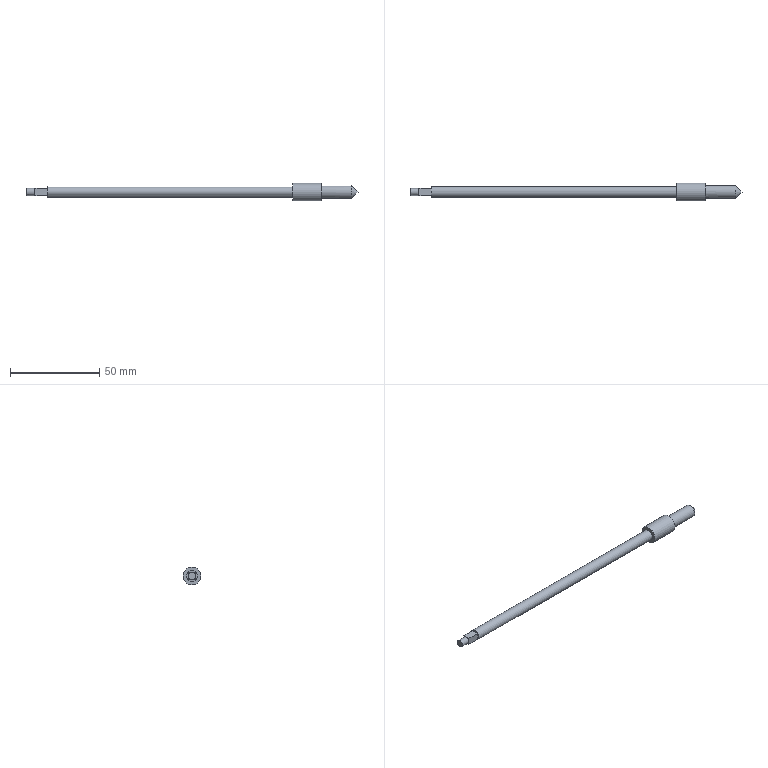Part | STEP file | 1-23.5 | 1 solid | 17 faces | box 185.5 x 10 x 10 mm | volume 6004 mm3 | plane 12 | cylinder 4 | cone 1 | commonest cylinder face diameters 4 x1 6 x1 7 x1 10 x1
STEP:
#1=CARTESIAN_POINT('',(0.,0.,0.));
#2=DIRECTION('',(0.,0.,1.));
#3=DIRECTION('',(1.,0.,0.));
#4=AXIS2_PLACEMENT_3D('',#1,#2,#3);
#5=CARTESIAN_POINT('',(0.,5.,0.));
#6=VERTEX_POINT('',#5);
#7=CARTESIAN_POINT('',(-16.,5.,0.));
#8=VERTEX_POINT('',#7);
#9=CARTESIAN_POINT('',(0.,5.,0.));
#10=DIRECTION('',(-1.,0.,0.));
#11=VECTOR('',#10,1.);
#12=LINE('',#9,#11);
#13=CARTESIAN_POINT('',(0.,0.,0.));
#14=DIRECTION('',(-1.,0.,0.));
#15=DIRECTION('',(0.,1.,0.));
#16=AXIS2_PLACEMENT_3D('',#13,#14,#15);
#17=CYLINDRICAL_SURFACE('',#16,5.);
#18=CARTESIAN_POINT('',(6.283,0.));
#19=DIRECTION('',(0.,1.));
#20=VECTOR('',#19,1.);
#21=LINE('',#18,#20);
#22=(GEOMETRIC_REPRESENTATION_CONTEXT(2)PARAMETRIC_REPRESENTATION_CONTEXT()REPRESENTATION_CONTEXT('',''));
#23=DEFINITIONAL_REPRESENTATION('',(#21),#22);
#24=PCURVE('',#17,#23);
#25=CARTESIAN_POINT('',(0.,0.));
#26=DIRECTION('',(0.,1.));
#27=VECTOR('',#26,1.);
#28=LINE('',#25,#27);
#29=(GEOMETRIC_REPRESENTATION_CONTEXT(2)PARAMETRIC_REPRESENTATION_CONTEXT()REPRESENTATION_CONTEXT('',''));
#30=DEFINITIONAL_REPRESENTATION('',(#28),#29);
#31=PCURVE('',#17,#30);
#32=SEAM_CURVE('',#12,(#24,#31),.PCURVE_S1.);
#33=EDGE_CURVE('',#6,#8,#32,.T.);
#34=ORIENTED_EDGE('',*,*,#33,.T.);
#35=CARTESIAN_POINT('',(-16.,0.,0.));
#36=DIRECTION('',(1.,0.,0.));
#37=DIRECTION('',(0.,1.,0.));
#38=AXIS2_PLACEMENT_3D('',#35,#36,#37);
#39=CIRCLE('',#38,5.);
#40=CARTESIAN_POINT('',(6.283,16.));
#41=DIRECTION('',(-1.,0.));
#42=VECTOR('',#41,1.);
#43=LINE('',#40,#42);
#44=(GEOMETRIC_REPRESENTATION_CONTEXT(2)PARAMETRIC_REPRESENTATION_CONTEXT()REPRESENTATION_CONTEXT('',''));
#45=DEFINITIONAL_REPRESENTATION('',(#43),#44);
#46=PCURVE('',#17,#45);
#47=CARTESIAN_POINT('',(-16.,-1.34,0.));
#48=DIRECTION('',(1.,0.,0.));
#49=DIRECTION('',(0.,0.,-1.));
#50=AXIS2_PLACEMENT_3D('',#47,#48,#49);
#51=PLANE('',#50);
#52=CARTESIAN_POINT('',(0.,1.34));
#53=DIRECTION('',(0.,1.));
#54=AXIS2_PLACEMENT_2D('',#52,#53);
#55=CIRCLE('',#54,5.);
#56=(GEOMETRIC_REPRESENTATION_CONTEXT(2)PARAMETRIC_REPRESENTATION_CONTEXT()REPRESENTATION_CONTEXT('',''));
#57=DEFINITIONAL_REPRESENTATION('',(#55),#56);
#58=PCURVE('',#51,#57);
#59=SURFACE_CURVE('',#39,(#46,#58),.PCURVE_S1.);
#60=EDGE_CURVE('',#8,#8,#59,.T.);
#61=ORIENTED_EDGE('',*,*,#60,.T.);
#62=ORIENTED_EDGE('',*,*,#33,.F.);
#63=CARTESIAN_POINT('',(0.,0.,0.));
#64=DIRECTION('',(1.,0.,0.));
#65=DIRECTION('',(0.,1.,0.));
#66=AXIS2_PLACEMENT_3D('',#63,#64,#65);
#67=CIRCLE('',#66,5.);
#68=CARTESIAN_POINT('',(6.283,0.));
#69=DIRECTION('',(-1.,0.));
#70=VECTOR('',#69,1.);
#71=LINE('',#68,#70);
#72=(GEOMETRIC_REPRESENTATION_CONTEXT(2)PARAMETRIC_REPRESENTATION_CONTEXT()REPRESENTATION_CONTEXT('',''));
#73=DEFINITIONAL_REPRESENTATION('',(#71),#72);
#74=PCURVE('',#17,#73);
#75=CARTESIAN_POINT('',(0.,-1.34,0.));
#76=DIRECTION('',(1.,0.,0.));
#77=DIRECTION('',(0.,0.,-1.));
#78=AXIS2_PLACEMENT_3D('',#75,#76,#77);
#79=PLANE('',#78);
#80=CARTESIAN_POINT('',(0.,1.34));
#81=DIRECTION('',(0.,1.));
#82=AXIS2_PLACEMENT_2D('',#80,#81);
#83=CIRCLE('',#82,5.);
#84=(GEOMETRIC_REPRESENTATION_CONTEXT(2)PARAMETRIC_REPRESENTATION_CONTEXT()REPRESENTATION_CONTEXT('',''));
#85=DEFINITIONAL_REPRESENTATION('',(#83),#84);
#86=PCURVE('',#79,#85);
#87=SURFACE_CURVE('',#67,(#74,#86),.PCURVE_S1.);
#88=EDGE_CURVE('',#6,#6,#87,.T.);
#89=ORIENTED_EDGE('',*,*,#88,.F.);
#90=EDGE_LOOP('',(#34,#61,#62,#89));
#91=FACE_BOUND('',#90,.T.);
#92=ADVANCED_FACE('',(#91),#17,.T.);
#93=ORIENTED_EDGE('',*,*,#88,.T.);
#94=EDGE_LOOP('',(#93));
#95=FACE_BOUND('',#94,.T.);
#96=CARTESIAN_POINT('',(0.,3.5,0.));
#97=VERTEX_POINT('',#96);
#98=CARTESIAN_POINT('',(0.,0.,0.));
#99=DIRECTION('',(1.,0.,0.));
#100=DIRECTION('',(0.,1.,0.));
#101=AXIS2_PLACEMENT_3D('',#98,#99,#100);
#102=CIRCLE('',#101,3.5);
#103=CARTESIAN_POINT('',(0.,1.34));
#104=DIRECTION('',(0.,1.));
#105=AXIS2_PLACEMENT_2D('',#103,#104);
#106=CIRCLE('',#105,3.5);
#107=(GEOMETRIC_REPRESENTATION_CONTEXT(2)PARAMETRIC_REPRESENTATION_CONTEXT()REPRESENTATION_CONTEXT('',''));
#108=DEFINITIONAL_REPRESENTATION('',(#106),#107);
#109=PCURVE('',#79,#108);
#110=CARTESIAN_POINT('',(0.,0.,0.));
#111=DIRECTION('',(1.,0.,0.));
#112=DIRECTION('',(0.,1.,0.));
#113=AXIS2_PLACEMENT_3D('',#110,#111,#112);
#114=CYLINDRICAL_SURFACE('',#113,3.5);
#115=CARTESIAN_POINT('',(0.,0.));
#116=DIRECTION('',(1.,0.));
#117=VECTOR('',#116,1.);
#118=LINE('',#115,#117);
#119=(GEOMETRIC_REPRESENTATION_CONTEXT(2)PARAMETRIC_REPRESENTATION_CONTEXT()REPRESENTATION_CONTEXT('',''));
#120=DEFINITIONAL_REPRESENTATION('',(#118),#119);
#121=PCURVE('',#114,#120);
#122=SURFACE_CURVE('',#102,(#109,#121),.PCURVE_S1.);
#123=EDGE_CURVE('',#97,#97,#122,.T.);
#124=ORIENTED_EDGE('',*,*,#123,.F.);
#125=EDGE_LOOP('',(#124));
#126=FACE_BOUND('',#125,.T.);
#127=ADVANCED_FACE('',(#95,#126),#79,.T.);
#128=ORIENTED_EDGE('',*,*,#123,.T.);
#129=CARTESIAN_POINT('',(17.,3.5,0.));
#130=VERTEX_POINT('',#129);
#131=CARTESIAN_POINT('',(0.,3.5,0.));
#132=DIRECTION('',(1.,0.,0.));
#133=VECTOR('',#132,1.);
#134=LINE('',#131,#133);
#135=CARTESIAN_POINT('',(6.283,0.));
#136=DIRECTION('',(0.,1.));
#137=VECTOR('',#136,1.);
#138=LINE('',#135,#137);
#139=(GEOMETRIC_REPRESENTATION_CONTEXT(2)PARAMETRIC_REPRESENTATION_CONTEXT()REPRESENTATION_CONTEXT('',''));
#140=DEFINITIONAL_REPRESENTATION('',(#138),#139);
#141=PCURVE('',#114,#140);
#142=CARTESIAN_POINT('',(0.,0.));
#143=DIRECTION('',(0.,1.));
#144=VECTOR('',#143,1.);
#145=LINE('',#142,#144);
#146=(GEOMETRIC_REPRESENTATION_CONTEXT(2)PARAMETRIC_REPRESENTATION_CONTEXT()REPRESENTATION_CONTEXT('',''));
#147=DEFINITIONAL_REPRESENTATION('',(#145),#146);
#148=PCURVE('',#114,#147);
#149=SEAM_CURVE('',#134,(#141,#148),.PCURVE_S1.);
#150=EDGE_CURVE('',#97,#130,#149,.T.);
#151=ORIENTED_EDGE('',*,*,#150,.T.);
#152=CARTESIAN_POINT('',(17.,0.,3.5));
#153=VERTEX_POINT('',#152);
#154=CARTESIAN_POINT('',(17.,0.,0.));
#155=DIRECTION('',(1.,0.,0.));
#156=DIRECTION('',(0.,0.,1.));
#157=AXIS2_PLACEMENT_3D('',#154,#155,#156);
#158=CIRCLE('',#157,3.5);
#159=CARTESIAN_POINT('',(1.571,17.));
#160=DIRECTION('',(1.,0.));
#161=VECTOR('',#160,1.);
#162=LINE('',#159,#161);
#163=(GEOMETRIC_REPRESENTATION_CONTEXT(2)PARAMETRIC_REPRESENTATION_CONTEXT()REPRESENTATION_CONTEXT('',''));
#164=DEFINITIONAL_REPRESENTATION('',(#162),#163);
#165=PCURVE('',#114,#164);
#166=CARTESIAN_POINT('',(20.5,0.,0.));
#167=DIRECTION('',(-1.,0.,0.));
#168=DIRECTION('',(0.,0.,1.));
#169=AXIS2_PLACEMENT_3D('',#166,#167,#168);
#170=CONICAL_SURFACE('',#169,0.,0.7854);
#171=CARTESIAN_POINT('',(6.283,3.5));
#172=DIRECTION('',(-1.,0.));
#173=VECTOR('',#172,1.);
#174=LINE('',#171,#173);
#175=(GEOMETRIC_REPRESENTATION_CONTEXT(2)PARAMETRIC_REPRESENTATION_CONTEXT()REPRESENTATION_CONTEXT('',''));
#176=DEFINITIONAL_REPRESENTATION('',(#174),#175);
#177=PCURVE('',#170,#176);
#178=SURFACE_CURVE('',#158,(#165,#177),.PCURVE_S1.);
#179=EDGE_CURVE('',#153,#130,#178,.T.);
#180=ORIENTED_EDGE('',*,*,#179,.F.);
#181=CARTESIAN_POINT('',(17.,0.,0.));
#182=DIRECTION('',(1.,0.,0.));
#183=DIRECTION('',(0.,1.,0.));
#184=AXIS2_PLACEMENT_3D('',#181,#182,#183);
#185=CIRCLE('',#184,3.5);
#186=CARTESIAN_POINT('',(0.,17.));
#187=DIRECTION('',(1.,0.));
#188=VECTOR('',#187,1.);
#189=LINE('',#186,#188);
#190=(GEOMETRIC_REPRESENTATION_CONTEXT(2)PARAMETRIC_REPRESENTATION_CONTEXT()REPRESENTATION_CONTEXT('',''));
#191=DEFINITIONAL_REPRESENTATION('',(#189),#190);
#192=PCURVE('',#114,#191);
#193=CARTESIAN_POINT('',(1.571,3.5));
#194=DIRECTION('',(-1.,0.));
#195=VECTOR('',#194,1.);
#196=LINE('',#193,#195);
#197=(GEOMETRIC_REPRESENTATION_CONTEXT(2)PARAMETRIC_REPRESENTATION_CONTEXT()REPRESENTATION_CONTEXT('',''));
#198=DEFINITIONAL_REPRESENTATION('',(#196),#197);
#199=PCURVE('',#170,#198);
#200=SURFACE_CURVE('',#185,(#192,#199),.PCURVE_S1.);
#201=EDGE_CURVE('',#130,#153,#200,.T.);
#202=ORIENTED_EDGE('',*,*,#201,.F.);
#203=ORIENTED_EDGE('',*,*,#150,.F.);
#204=EDGE_LOOP('',(#128,#151,#180,#202,#203));
#205=FACE_BOUND('',#204,.T.);
#206=ADVANCED_FACE('',(#205),#114,.T.);
#207=ORIENTED_EDGE('',*,*,#60,.T.);
#208=EDGE_LOOP('',(#207));
#209=FACE_BOUND('',#208,.F.);
#210=CARTESIAN_POINT('',(-16.,-3.,0.));
#211=VERTEX_POINT('',#210);
#212=CARTESIAN_POINT('',(-16.,0.,0.));
#213=DIRECTION('',(-1.,0.,0.));
#214=DIRECTION('',(0.,-1.,0.));
#215=AXIS2_PLACEMENT_3D('',#212,#213,#214);
#216=CIRCLE('',#215,3.);
#217=CARTESIAN_POINT('',(0.,-1.66));
#218=CARTESIAN_POINT('',(-5.196,-1.66));
#219=CARTESIAN_POINT('',(-2.598,2.84));
#220=CARTESIAN_POINT('',(0.,7.34));
#221=CARTESIAN_POINT('',(2.598,2.84));
#222=CARTESIAN_POINT('',(5.196,-1.66));
#223=CARTESIAN_POINT('',(0.,-1.66));
#224=(BOUNDED_CURVE()B_SPLINE_CURVE(2,(#217,#218,#219,#220,#221,#222,#223),.UNSPECIFIED.,.T.,.F.)B_SPLINE_CURVE_WITH_KNOTS((1,2,2,2,2,1),(-2.094,0.,2.094,4.189,6.283,8.378),.UNSPECIFIED.)CURVE()GEOMETRIC_REPRESENTATION_ITEM()RATIONAL_B_SPLINE_CURVE((1.,0.5,1.,0.5,1.,0.5,1.))REPRESENTATION_ITEM(''));
#225=(GEOMETRIC_REPRESENTATION_CONTEXT(2)PARAMETRIC_REPRESENTATION_CONTEXT()REPRESENTATION_CONTEXT('',''));
#226=DEFINITIONAL_REPRESENTATION('',(#224),#225);
#227=PCURVE('',#51,#226);
#228=CARTESIAN_POINT('',(-16.,0.,0.));
#229=DIRECTION('',(-1.,0.,0.));
#230=DIRECTION('',(0.,-1.,0.));
#231=AXIS2_PLACEMENT_3D('',#228,#229,#230);
#232=CYLINDRICAL_SURFACE('',#231,3.);
#233=CARTESIAN_POINT('',(0.,0.));
#234=DIRECTION('',(1.,0.));
#235=VECTOR('',#234,1.);
#236=LINE('',#233,#235);
#237=(GEOMETRIC_REPRESENTATION_CONTEXT(2)PARAMETRIC_REPRESENTATION_CONTEXT()REPRESENTATION_CONTEXT('',''));
#238=DEFINITIONAL_REPRESENTATION('',(#236),#237);
#239=PCURVE('',#232,#238);
#240=SURFACE_CURVE('',#216,(#227,#239),.PCURVE_S1.);
#241=EDGE_CURVE('',#211,#211,#240,.T.);
#242=ORIENTED_EDGE('',*,*,#241,.T.);
#243=EDGE_LOOP('',(#242));
#244=FACE_BOUND('',#243,.F.);
#245=ADVANCED_FACE('',(#209,#244),#51,.F.);
#246=ORIENTED_EDGE('',*,*,#241,.T.);
#247=CARTESIAN_POINT('',(-153.,-3.,0.));
#248=VERTEX_POINT('',#247);
#249=CARTESIAN_POINT('',(-16.,-3.,0.));
#250=DIRECTION('',(-1.,0.,0.));
#251=VECTOR('',#250,1.);
#252=LINE('',#249,#251);
#253=CARTESIAN_POINT('',(6.283,0.));
#254=DIRECTION('',(0.,1.));
#255=VECTOR('',#254,1.);
#256=LINE('',#253,#255);
#257=(GEOMETRIC_REPRESENTATION_CONTEXT(2)PARAMETRIC_REPRESENTATION_CONTEXT()REPRESENTATION_CONTEXT('',''));
#258=DEFINITIONAL_REPRESENTATION('',(#256),#257);
#259=PCURVE('',#232,#258);
#260=CARTESIAN_POINT('',(0.,0.));
#261=DIRECTION('',(0.,1.));
#262=VECTOR('',#261,1.);
#263=LINE('',#260,#262);
#264=(GEOMETRIC_REPRESENTATION_CONTEXT(2)PARAMETRIC_REPRESENTATION_CONTEXT()REPRESENTATION_CONTEXT('',''));
#265=DEFINITIONAL_REPRESENTATION('',(#263),#264);
#266=PCURVE('',#232,#265);
#267=SEAM_CURVE('',#252,(#259,#266),.PCURVE_S1.);
#268=EDGE_CURVE('',#211,#248,#267,.T.);
#269=ORIENTED_EDGE('',*,*,#268,.T.);
#270=CARTESIAN_POINT('',(-153.,0.,0.));
#271=DIRECTION('',(-1.,0.,0.));
#272=DIRECTION('',(0.,-1.,0.));
#273=AXIS2_PLACEMENT_3D('',#270,#271,#272);
#274=CIRCLE('',#273,3.);
#275=CARTESIAN_POINT('',(0.,137.));
#276=DIRECTION('',(1.,0.));
#277=VECTOR('',#276,1.);
#278=LINE('',#275,#277);
#279=(GEOMETRIC_REPRESENTATION_CONTEXT(2)PARAMETRIC_REPRESENTATION_CONTEXT()REPRESENTATION_CONTEXT('',''));
#280=DEFINITIONAL_REPRESENTATION('',(#278),#279);
#281=PCURVE('',#232,#280);
#282=CARTESIAN_POINT('',(-153.,0.8038,0.));
#283=DIRECTION('',(-1.,0.,0.));
#284=DIRECTION('',(0.,-1.,0.));
#285=AXIS2_PLACEMENT_3D('',#282,#283,#284);
#286=PLANE('',#285);
#287=CARTESIAN_POINT('',(0.8038,0.));
#288=DIRECTION('',(1.,0.));
#289=AXIS2_PLACEMENT_2D('',#287,#288);
#290=CIRCLE('',#289,3.);
#291=(GEOMETRIC_REPRESENTATION_CONTEXT(2)PARAMETRIC_REPRESENTATION_CONTEXT()REPRESENTATION_CONTEXT('',''));
#292=DEFINITIONAL_REPRESENTATION('',(#290),#291);
#293=PCURVE('',#286,#292);
#294=SURFACE_CURVE('',#274,(#281,#293),.PCURVE_S1.);
#295=EDGE_CURVE('',#248,#248,#294,.T.);
#296=ORIENTED_EDGE('',*,*,#295,.F.);
#297=ORIENTED_EDGE('',*,*,#268,.F.);
#298=EDGE_LOOP('',(#246,#269,#296,#297));
#299=FACE_BOUND('',#298,.T.);
#300=ADVANCED_FACE('',(#299),#232,.T.);
#301=ORIENTED_EDGE('',*,*,#295,.T.);
#302=EDGE_LOOP('',(#301));
#303=FACE_BOUND('',#302,.T.);
#304=CARTESIAN_POINT('',(-153.,-2.,-2.));
#305=VERTEX_POINT('',#304);
#306=CARTESIAN_POINT('',(-153.,-2.,2.));
#307=VERTEX_POINT('',#306);
#308=CARTESIAN_POINT('',(-153.,-2.,-2.));
#309=DIRECTION('',(0.,0.,1.));
#310=VECTOR('',#309,1.);
#311=LINE('',#308,#310);
#312=CARTESIAN_POINT('',(2.804,-2.));
#313=DIRECTION('',(0.,1.));
#314=VECTOR('',#313,1.);
#315=LINE('',#312,#314);
#316=(GEOMETRIC_REPRESENTATION_CONTEXT(2)PARAMETRIC_REPRESENTATION_CONTEXT()REPRESENTATION_CONTEXT('',''));
#317=DEFINITIONAL_REPRESENTATION('',(#315),#316);
#318=PCURVE('',#286,#317);
#319=CARTESIAN_POINT('',(-156.5,-2.,0.));
#320=DIRECTION('',(0.,-1.,0.));
#321=DIRECTION('',(0.,0.,1.));
#322=AXIS2_PLACEMENT_3D('',#319,#320,#321);
#323=PLANE('',#322);
#324=CARTESIAN_POINT('',(-2.,-3.5));
#325=DIRECTION('',(1.,0.));
#326=VECTOR('',#325,1.);
#327=LINE('',#324,#326);
#328=(GEOMETRIC_REPRESENTATION_CONTEXT(2)PARAMETRIC_REPRESENTATION_CONTEXT()REPRESENTATION_CONTEXT('',''));
#329=DEFINITIONAL_REPRESENTATION('',(#327),#328);
#330=PCURVE('',#323,#329);
#331=SURFACE_CURVE('',#311,(#318,#330),.PCURVE_S1.);
#332=EDGE_CURVE('',#305,#307,#331,.T.);
#333=ORIENTED_EDGE('',*,*,#332,.F.);
#334=CARTESIAN_POINT('',(-153.,2.,-2.));
#335=VERTEX_POINT('',#334);
#336=CARTESIAN_POINT('',(-153.,2.,-2.));
#337=DIRECTION('',(0.,-1.,0.));
#338=VECTOR('',#337,1.);
#339=LINE('',#336,#338);
#340=CARTESIAN_POINT('',(-1.196,-2.));
#341=DIRECTION('',(1.,0.));
#342=VECTOR('',#341,1.);
#343=LINE('',#340,#342);
#344=(GEOMETRIC_REPRESENTATION_CONTEXT(2)PARAMETRIC_REPRESENTATION_CONTEXT()REPRESENTATION_CONTEXT('',''));
#345=DEFINITIONAL_REPRESENTATION('',(#343),#344);
#346=PCURVE('',#286,#345);
#347=CARTESIAN_POINT('',(-156.5,0.,-2.));
#348=DIRECTION('',(0.,0.,-1.));
#349=DIRECTION('',(0.,-1.,0.));
#350=AXIS2_PLACEMENT_3D('',#347,#348,#349);
#351=PLANE('',#350);
#352=CARTESIAN_POINT('',(-2.,-3.5));
#353=DIRECTION('',(1.,0.));
#354=VECTOR('',#353,1.);
#355=LINE('',#352,#354);
#356=(GEOMETRIC_REPRESENTATION_CONTEXT(2)PARAMETRIC_REPRESENTATION_CONTEXT()REPRESENTATION_CONTEXT('',''));
#357=DEFINITIONAL_REPRESENTATION('',(#355),#356);
#358=PCURVE('',#351,#357);
#359=SURFACE_CURVE('',#339,(#346,#358),.PCURVE_S1.);
#360=EDGE_CURVE('',#335,#305,#359,.T.);
#361=ORIENTED_EDGE('',*,*,#360,.F.);
#362=CARTESIAN_POINT('',(-153.,2.,2.));
#363=VERTEX_POINT('',#362);
#364=CARTESIAN_POINT('',(-153.,2.,2.));
#365=DIRECTION('',(0.,0.,-1.));
#366=VECTOR('',#365,1.);
#367=LINE('',#364,#366);
#368=CARTESIAN_POINT('',(-1.196,2.));
#369=DIRECTION('',(0.,-1.));
#370=VECTOR('',#369,1.);
#371=LINE('',#368,#370);
#372=(GEOMETRIC_REPRESENTATION_CONTEXT(2)PARAMETRIC_REPRESENTATION_CONTEXT()REPRESENTATION_CONTEXT('',''));
#373=DEFINITIONAL_REPRESENTATION('',(#371),#372);
#374=PCURVE('',#286,#373);
#375=CARTESIAN_POINT('',(-156.5,2.,0.));
#376=DIRECTION('',(0.,1.,0.));
#377=DIRECTION('',(0.,0.,-1.));
#378=AXIS2_PLACEMENT_3D('',#375,#376,#377);
#379=PLANE('',#378);
#380=CARTESIAN_POINT('',(-2.,-3.5));
#381=DIRECTION('',(1.,0.));
#382=VECTOR('',#381,1.);
#383=LINE('',#380,#382);
#384=(GEOMETRIC_REPRESENTATION_CONTEXT(2)PARAMETRIC_REPRESENTATION_CONTEXT()REPRESENTATION_CONTEXT('',''));
#385=DEFINITIONAL_REPRESENTATION('',(#383),#384);
#386=PCURVE('',#379,#385);
#387=SURFACE_CURVE('',#367,(#374,#386),.PCURVE_S1.);
#388=EDGE_CURVE('',#363,#335,#387,.T.);
#389=ORIENTED_EDGE('',*,*,#388,.F.);
#390=CARTESIAN_POINT('',(-153.,-2.,2.));
#391=DIRECTION('',(0.,1.,0.));
#392=VECTOR('',#391,1.);
#393=LINE('',#390,#392);
#394=CARTESIAN_POINT('',(2.804,2.));
#395=DIRECTION('',(-1.,0.));
#396=VECTOR('',#395,1.);
#397=LINE('',#394,#396);
#398=(GEOMETRIC_REPRESENTATION_CONTEXT(2)PARAMETRIC_REPRESENTATION_CONTEXT()REPRESENTATION_CONTEXT('',''));
#399=DEFINITIONAL_REPRESENTATION('',(#397),#398);
#400=PCURVE('',#286,#399);
#401=CARTESIAN_POINT('',(-156.5,0.,2.));
#402=DIRECTION('',(0.,0.,1.));
#403=DIRECTION('',(0.,1.,0.));
#404=AXIS2_PLACEMENT_3D('',#401,#402,#403);
#405=PLANE('',#404);
#406=CARTESIAN_POINT('',(-2.,-3.5));
#407=DIRECTION('',(1.,0.));
#408=VECTOR('',#407,1.);
#409=LINE('',#406,#408);
#410=(GEOMETRIC_REPRESENTATION_CONTEXT(2)PARAMETRIC_REPRESENTATION_CONTEXT()REPRESENTATION_CONTEXT('',''));
#411=DEFINITIONAL_REPRESENTATION('',(#409),#410);
#412=PCURVE('',#405,#411);
#413=SURFACE_CURVE('',#393,(#400,#412),.PCURVE_S1.);
#414=EDGE_CURVE('',#307,#363,#413,.T.);
#415=ORIENTED_EDGE('',*,*,#414,.F.);
#416=EDGE_LOOP('',(#333,#361,#389,#415));
#417=FACE_BOUND('',#416,.T.);
#418=ADVANCED_FACE('',(#303,#417),#286,.T.);
#419=ORIENTED_EDGE('',*,*,#332,.T.);
#420=CARTESIAN_POINT('',(-160.,-2.,2.));
#421=VERTEX_POINT('',#420);
#422=CARTESIAN_POINT('',(-153.,-2.,2.));
#423=DIRECTION('',(-1.,0.,0.));
#424=VECTOR('',#423,1.);
#425=LINE('',#422,#424);
#426=CARTESIAN_POINT('',(2.,-3.5));
#427=DIRECTION('',(0.,1.));
#428=VECTOR('',#427,1.);
#429=LINE('',#426,#428);
#430=(GEOMETRIC_REPRESENTATION_CONTEXT(2)PARAMETRIC_REPRESENTATION_CONTEXT()REPRESENTATION_CONTEXT('',''));
#431=DEFINITIONAL_REPRESENTATION('',(#429),#430);
#432=PCURVE('',#323,#431);
#433=CARTESIAN_POINT('',(-2.,-3.5));
#434=DIRECTION('',(0.,1.));
#435=VECTOR('',#434,1.);
#436=LINE('',#433,#435);
#437=(GEOMETRIC_REPRESENTATION_CONTEXT(2)PARAMETRIC_REPRESENTATION_CONTEXT()REPRESENTATION_CONTEXT('',''));
#438=DEFINITIONAL_REPRESENTATION('',(#436),#437);
#439=PCURVE('',#405,#438);
#440=SURFACE_CURVE('',#425,(#432,#439),.PCURVE_S1.);
#441=EDGE_CURVE('',#307,#421,#440,.T.);
#442=ORIENTED_EDGE('',*,*,#441,.T.);
#443=CARTESIAN_POINT('',(-160.,-2.,0.));
#444=VERTEX_POINT('',#443);
#445=CARTESIAN_POINT('',(-160.,-2.,0.));
#446=DIRECTION('',(0.,0.,1.));
#447=VECTOR('',#446,1.);
#448=LINE('',#445,#447);
#449=CARTESIAN_POINT('',(0.,3.5));
#450=DIRECTION('',(1.,0.));
#451=VECTOR('',#450,1.);
#452=LINE('',#449,#451);
#453=(GEOMETRIC_REPRESENTATION_CONTEXT(2)PARAMETRIC_REPRESENTATION_CONTEXT()REPRESENTATION_CONTEXT('',''));
#454=DEFINITIONAL_REPRESENTATION('',(#452),#453);
#455=PCURVE('',#323,#454);
#456=CARTESIAN_POINT('',(-160.,0.,0.));
#457=DIRECTION('',(-1.,0.,0.));
#458=DIRECTION('',(0.,-1.,0.));
#459=AXIS2_PLACEMENT_3D('',#456,#457,#458);
#460=PLANE('',#459);
#461=CARTESIAN_POINT('',(2.,0.));
#462=DIRECTION('',(0.,1.));
#463=VECTOR('',#462,1.);
#464=LINE('',#461,#463);
#465=(GEOMETRIC_REPRESENTATION_CONTEXT(2)PARAMETRIC_REPRESENTATION_CONTEXT()REPRESENTATION_CONTEXT('',''));
#466=DEFINITIONAL_REPRESENTATION('',(#464),#465);
#467=PCURVE('',#460,#466);
#468=SURFACE_CURVE('',#448,(#455,#467),.PCURVE_S1.);
#469=EDGE_CURVE('',#444,#421,#468,.T.);
#470=ORIENTED_EDGE('',*,*,#469,.F.);
#471=CARTESIAN_POINT('',(-160.,-2.,-2.));
#472=VERTEX_POINT('',#471);
#473=CARTESIAN_POINT('',(-160.,-2.,-2.));
#474=DIRECTION('',(0.,0.,1.));
#475=VECTOR('',#474,1.);
#476=LINE('',#473,#475);
#477=CARTESIAN_POINT('',(-2.,3.5));
#478=DIRECTION('',(1.,0.));
#479=VECTOR('',#478,1.);
#480=LINE('',#477,#479);
#481=(GEOMETRIC_REPRESENTATION_CONTEXT(2)PARAMETRIC_REPRESENTATION_CONTEXT()REPRESENTATION_CONTEXT('',''));
#482=DEFINITIONAL_REPRESENTATION('',(#480),#481);
#483=PCURVE('',#323,#482);
#484=CARTESIAN_POINT('',(-160.,0.,0.));
#485=DIRECTION('',(-1.,0.,0.));
#486=DIRECTION('',(0.,-1.,0.));
#487=AXIS2_PLACEMENT_3D('',#484,#485,#486);
#488=PLANE('',#487);
#489=CARTESIAN_POINT('',(2.,-2.));
#490=DIRECTION('',(0.,1.));
#491=VECTOR('',#490,1.);
#492=LINE('',#489,#491);
#493=(GEOMETRIC_REPRESENTATION_CONTEXT(2)PARAMETRIC_REPRESENTATION_CONTEXT()REPRESENTATION_CONTEXT('',''));
#494=DEFINITIONAL_REPRESENTATION('',(#492),#493);
#495=PCURVE('',#488,#494);
#496=SURFACE_CURVE('',#476,(#483,#495),.PCURVE_S1.);
#497=EDGE_CURVE('',#472,#444,#496,.T.);
#498=ORIENTED_EDGE('',*,*,#497,.F.);
#499=CARTESIAN_POINT('',(-153.,-2.,-2.));
#500=DIRECTION('',(-1.,0.,0.));
#501=VECTOR('',#500,1.);
#502=LINE('',#499,#501);
#503=CARTESIAN_POINT('',(-2.,-3.5));
#504=DIRECTION('',(0.,1.));
#505=VECTOR('',#504,1.);
#506=LINE('',#503,#505);
#507=(GEOMETRIC_REPRESENTATION_CONTEXT(2)PARAMETRIC_REPRESENTATION_CONTEXT()REPRESENTATION_CONTEXT('',''));
#508=DEFINITIONAL_REPRESENTATION('',(#506),#507);
#509=PCURVE('',#323,#508);
#510=CARTESIAN_POINT('',(2.,-3.5));
#511=DIRECTION('',(0.,1.));
#512=VECTOR('',#511,1.);
#513=LINE('',#510,#512);
#514=(GEOMETRIC_REPRESENTATION_CONTEXT(2)PARAMETRIC_REPRESENTATION_CONTEXT()REPRESENTATION_CONTEXT('',''));
#515=DEFINITIONAL_REPRESENTATION('',(#513),#514);
#516=PCURVE('',#351,#515);
#517=SURFACE_CURVE('',#502,(#509,#516),.PCURVE_S1.);
#518=EDGE_CURVE('',#305,#472,#517,.T.);
#519=ORIENTED_EDGE('',*,*,#518,.F.);
#520=EDGE_LOOP('',(#419,#442,#470,#498,#519));
#521=FACE_BOUND('',#520,.T.);
#522=ADVANCED_FACE('',(#521),#323,.T.);
#523=ORIENTED_EDGE('',*,*,#360,.T.);
#524=ORIENTED_EDGE('',*,*,#518,.T.);
#525=CARTESIAN_POINT('',(-160.,0.,-2.));
#526=VERTEX_POINT('',#525);
#527=CARTESIAN_POINT('',(-160.,0.,-2.));
#528=DIRECTION('',(0.,-1.,0.));
#529=VECTOR('',#528,1.);
#530=LINE('',#527,#529);
#531=CARTESIAN_POINT('',(0.,3.5));
#532=DIRECTION('',(1.,0.));
#533=VECTOR('',#532,1.);
#534=LINE('',#531,#533);
#535=(GEOMETRIC_REPRESENTATION_CONTEXT(2)PARAMETRIC_REPRESENTATION_CONTEXT()REPRESENTATION_CONTEXT('',''));
#536=DEFINITIONAL_REPRESENTATION('',(#534),#535);
#537=PCURVE('',#351,#536);
#538=CARTESIAN_POINT('',(0.,-2.));
#539=DIRECTION('',(1.,0.));
#540=VECTOR('',#539,1.);
#541=LINE('',#538,#540);
#542=(GEOMETRIC_REPRESENTATION_CONTEXT(2)PARAMETRIC_REPRESENTATION_CONTEXT()REPRESENTATION_CONTEXT('',''));
#543=DEFINITIONAL_REPRESENTATION('',(#541),#542);
#544=PCURVE('',#488,#543);
#545=SURFACE_CURVE('',#530,(#537,#544),.PCURVE_S1.);
#546=EDGE_CURVE('',#526,#472,#545,.T.);
#547=ORIENTED_EDGE('',*,*,#546,.F.);
#548=CARTESIAN_POINT('',(-160.,2.,-2.));
#549=VERTEX_POINT('',#548);
#550=CARTESIAN_POINT('',(-160.,2.,-2.));
#551=DIRECTION('',(0.,-1.,0.));
#552=VECTOR('',#551,1.);
#553=LINE('',#550,#552);
#554=CARTESIAN_POINT('',(-2.,3.5));
#555=DIRECTION('',(1.,0.));
#556=VECTOR('',#555,1.);
#557=LINE('',#554,#556);
#558=(GEOMETRIC_REPRESENTATION_CONTEXT(2)PARAMETRIC_REPRESENTATION_CONTEXT()REPRESENTATION_CONTEXT('',''));
#559=DEFINITIONAL_REPRESENTATION('',(#557),#558);
#560=PCURVE('',#351,#559);
#561=CARTESIAN_POINT('',(-160.,0.,0.));
#562=DIRECTION('',(-1.,0.,0.));
#563=DIRECTION('',(0.,-1.,0.));
#564=AXIS2_PLACEMENT_3D('',#561,#562,#563);
#565=PLANE('',#564);
#566=CARTESIAN_POINT('',(-2.,-2.));
#567=DIRECTION('',(1.,0.));
#568=VECTOR('',#567,1.);
#569=LINE('',#566,#568);
#570=(GEOMETRIC_REPRESENTATION_CONTEXT(2)PARAMETRIC_REPRESENTATION_CONTEXT()REPRESENTATION_CONTEXT('',''));
#571=DEFINITIONAL_REPRESENTATION('',(#569),#570);
#572=PCURVE('',#565,#571);
#573=SURFACE_CURVE('',#553,(#560,#572),.PCURVE_S1.);
#574=EDGE_CURVE('',#549,#526,#573,.T.);
#575=ORIENTED_EDGE('',*,*,#574,.F.);
#576=CARTESIAN_POINT('',(-153.,2.,-2.));
#577=DIRECTION('',(-1.,0.,0.));
#578=VECTOR('',#577,1.);
#579=LINE('',#576,#578);
#580=CARTESIAN_POINT('',(-2.,-3.5));
#581=DIRECTION('',(0.,1.));
#582=VECTOR('',#581,1.);
#583=LINE('',#580,#582);
#584=(GEOMETRIC_REPRESENTATION_CONTEXT(2)PARAMETRIC_REPRESENTATION_CONTEXT()REPRESENTATION_CONTEXT('',''));
#585=DEFINITIONAL_REPRESENTATION('',(#583),#584);
#586=PCURVE('',#351,#585);
#587=CARTESIAN_POINT('',(2.,-3.5));
#588=DIRECTION('',(0.,1.));
#589=VECTOR('',#588,1.);
#590=LINE('',#587,#589);
#591=(GEOMETRIC_REPRESENTATION_CONTEXT(2)PARAMETRIC_REPRESENTATION_CONTEXT()REPRESENTATION_CONTEXT('',''));
#592=DEFINITIONAL_REPRESENTATION('',(#590),#591);
#593=PCURVE('',#379,#592);
#594=SURFACE_CURVE('',#579,(#586,#593),.PCURVE_S1.);
#595=EDGE_CURVE('',#335,#549,#594,.T.);
#596=ORIENTED_EDGE('',*,*,#595,.F.);
#597=EDGE_LOOP('',(#523,#524,#547,#575,#596));
#598=FACE_BOUND('',#597,.T.);
#599=ADVANCED_FACE('',(#598),#351,.T.);
#600=ORIENTED_EDGE('',*,*,#388,.T.);
#601=ORIENTED_EDGE('',*,*,#595,.T.);
#602=CARTESIAN_POINT('',(-160.,2.,0.));
#603=VERTEX_POINT('',#602);
#604=CARTESIAN_POINT('',(-160.,2.,0.));
#605=DIRECTION('',(0.,0.,-1.));
#606=VECTOR('',#605,1.);
#607=LINE('',#604,#606);
#608=CARTESIAN_POINT('',(0.,3.5));
#609=DIRECTION('',(1.,0.));
#610=VECTOR('',#609,1.);
#611=LINE('',#608,#610);
#612=(GEOMETRIC_REPRESENTATION_CONTEXT(2)PARAMETRIC_REPRESENTATION_CONTEXT()REPRESENTATION_CONTEXT('',''));
#613=DEFINITIONAL_REPRESENTATION('',(#611),#612);
#614=PCURVE('',#379,#613);
#615=CARTESIAN_POINT('',(-2.,0.));
#616=DIRECTION('',(0.,-1.));
#617=VECTOR('',#616,1.);
#618=LINE('',#615,#617);
#619=(GEOMETRIC_REPRESENTATION_CONTEXT(2)PARAMETRIC_REPRESENTATION_CONTEXT()REPRESENTATION_CONTEXT('',''));
#620=DEFINITIONAL_REPRESENTATION('',(#618),#619);
#621=PCURVE('',#565,#620);
#622=SURFACE_CURVE('',#607,(#614,#621),.PCURVE_S1.);
#623=EDGE_CURVE('',#603,#549,#622,.T.);
#624=ORIENTED_EDGE('',*,*,#623,.F.);
#625=CARTESIAN_POINT('',(-160.,2.,2.));
#626=VERTEX_POINT('',#625);
#627=CARTESIAN_POINT('',(-160.,2.,2.));
#628=DIRECTION('',(0.,0.,-1.));
#629=VECTOR('',#628,1.);
#630=LINE('',#627,#629);
#631=CARTESIAN_POINT('',(-2.,3.5));
#632=DIRECTION('',(1.,0.));
#633=VECTOR('',#632,1.);
#634=LINE('',#631,#633);
#635=(GEOMETRIC_REPRESENTATION_CONTEXT(2)PARAMETRIC_REPRESENTATION_CONTEXT()REPRESENTATION_CONTEXT('',''));
#636=DEFINITIONAL_REPRESENTATION('',(#634),#635);
#637=PCURVE('',#379,#636);
#638=CARTESIAN_POINT('',(-160.,0.,0.));
#639=DIRECTION('',(-1.,0.,0.));
#640=DIRECTION('',(0.,-1.,0.));
#641=AXIS2_PLACEMENT_3D('',#638,#639,#640);
#642=PLANE('',#641);
#643=CARTESIAN_POINT('',(-2.,2.));
#644=DIRECTION('',(0.,-1.));
#645=VECTOR('',#644,1.);
#646=LINE('',#643,#645);
#647=(GEOMETRIC_REPRESENTATION_CONTEXT(2)PARAMETRIC_REPRESENTATION_CONTEXT()REPRESENTATION_CONTEXT('',''));
#648=DEFINITIONAL_REPRESENTATION('',(#646),#647);
#649=PCURVE('',#642,#648);
#650=SURFACE_CURVE('',#630,(#637,#649),.PCURVE_S1.);
#651=EDGE_CURVE('',#626,#603,#650,.T.);
#652=ORIENTED_EDGE('',*,*,#651,.F.);
#653=CARTESIAN_POINT('',(-153.,2.,2.));
#654=DIRECTION('',(-1.,0.,0.));
#655=VECTOR('',#654,1.);
#656=LINE('',#653,#655);
#657=CARTESIAN_POINT('',(-2.,-3.5));
#658=DIRECTION('',(0.,1.));
#659=VECTOR('',#658,1.);
#660=LINE('',#657,#659);
#661=(GEOMETRIC_REPRESENTATION_CONTEXT(2)PARAMETRIC_REPRESENTATION_CONTEXT()REPRESENTATION_CONTEXT('',''));
#662=DEFINITIONAL_REPRESENTATION('',(#660),#661);
#663=PCURVE('',#379,#662);
#664=CARTESIAN_POINT('',(2.,-3.5));
#665=DIRECTION('',(0.,1.));
#666=VECTOR('',#665,1.);
#667=LINE('',#664,#666);
#668=(GEOMETRIC_REPRESENTATION_CONTEXT(2)PARAMETRIC_REPRESENTATION_CONTEXT()REPRESENTATION_CONTEXT('',''));
#669=DEFINITIONAL_REPRESENTATION('',(#667),#668);
#670=PCURVE('',#405,#669);
#671=SURFACE_CURVE('',#656,(#663,#670),.PCURVE_S1.);
#672=EDGE_CURVE('',#363,#626,#671,.T.);
#673=ORIENTED_EDGE('',*,*,#672,.F.);
#674=EDGE_LOOP('',(#600,#601,#624,#652,#673));
#675=FACE_BOUND('',#674,.T.);
#676=ADVANCED_FACE('',(#675),#379,.T.);
#677=ORIENTED_EDGE('',*,*,#414,.T.);
#678=ORIENTED_EDGE('',*,*,#672,.T.);
#679=CARTESIAN_POINT('',(-160.,0.,2.));
#680=VERTEX_POINT('',#679);
#681=CARTESIAN_POINT('',(-160.,0.,2.));
#682=DIRECTION('',(0.,1.,0.));
#683=VECTOR('',#682,1.);
#684=LINE('',#681,#683);
#685=CARTESIAN_POINT('',(0.,3.5));
#686=DIRECTION('',(1.,0.));
#687=VECTOR('',#686,1.);
#688=LINE('',#685,#687);
#689=(GEOMETRIC_REPRESENTATION_CONTEXT(2)PARAMETRIC_REPRESENTATION_CONTEXT()REPRESENTATION_CONTEXT('',''));
#690=DEFINITIONAL_REPRESENTATION('',(#688),#689);
#691=PCURVE('',#405,#690);
#692=CARTESIAN_POINT('',(0.,2.));
#693=DIRECTION('',(-1.,0.));
#694=VECTOR('',#693,1.);
#695=LINE('',#692,#694);
#696=(GEOMETRIC_REPRESENTATION_CONTEXT(2)PARAMETRIC_REPRESENTATION_CONTEXT()REPRESENTATION_CONTEXT('',''));
#697=DEFINITIONAL_REPRESENTATION('',(#695),#696);
#698=PCURVE('',#642,#697);
#699=SURFACE_CURVE('',#684,(#691,#698),.PCURVE_S1.);
#700=EDGE_CURVE('',#680,#626,#699,.T.);
#701=ORIENTED_EDGE('',*,*,#700,.F.);
#702=CARTESIAN_POINT('',(-160.,-2.,2.));
#703=DIRECTION('',(0.,1.,0.));
#704=VECTOR('',#703,1.);
#705=LINE('',#702,#704);
#706=CARTESIAN_POINT('',(-2.,3.5));
#707=DIRECTION('',(1.,0.));
#708=VECTOR('',#707,1.);
#709=LINE('',#706,#708);
#710=(GEOMETRIC_REPRESENTATION_CONTEXT(2)PARAMETRIC_REPRESENTATION_CONTEXT()REPRESENTATION_CONTEXT('',''));
#711=DEFINITIONAL_REPRESENTATION('',(#709),#710);
#712=PCURVE('',#405,#711);
#713=CARTESIAN_POINT('',(2.,2.));
#714=DIRECTION('',(-1.,0.));
#715=VECTOR('',#714,1.);
#716=LINE('',#713,#715);
#717=(GEOMETRIC_REPRESENTATION_CONTEXT(2)PARAMETRIC_REPRESENTATION_CONTEXT()REPRESENTATION_CONTEXT('',''));
#718=DEFINITIONAL_REPRESENTATION('',(#716),#717);
#719=PCURVE('',#460,#718);
#720=SURFACE_CURVE('',#705,(#712,#719),.PCURVE_S1.);
#721=EDGE_CURVE('',#421,#680,#720,.T.);
#722=ORIENTED_EDGE('',*,*,#721,.F.);
#723=ORIENTED_EDGE('',*,*,#441,.F.);
#724=EDGE_LOOP('',(#677,#678,#701,#722,#723));
#725=FACE_BOUND('',#724,.T.);
#726=ADVANCED_FACE('',(#725),#405,.T.);
#727=ORIENTED_EDGE('',*,*,#574,.T.);
#728=CARTESIAN_POINT('',(-160.,0.,0.));
#729=DIRECTION('',(-1.,0.,0.));
#730=DIRECTION('',(0.,1.,0.));
#731=AXIS2_PLACEMENT_3D('',#728,#729,#730);
#732=CIRCLE('',#731,2.);
#733=CARTESIAN_POINT('',(0.,0.));
#734=DIRECTION('',(-1.,0.));
#735=AXIS2_PLACEMENT_2D('',#733,#734);
#736=CIRCLE('',#735,2.);
#737=(GEOMETRIC_REPRESENTATION_CONTEXT(2)PARAMETRIC_REPRESENTATION_CONTEXT()REPRESENTATION_CONTEXT('',''));
#738=DEFINITIONAL_REPRESENTATION('',(#736),#737);
#739=PCURVE('',#565,#738);
#740=CARTESIAN_POINT('',(-160.,0.,0.));
#741=DIRECTION('',(-1.,0.,0.));
#742=DIRECTION('',(0.,-1.,0.));
#743=AXIS2_PLACEMENT_3D('',#740,#741,#742);
#744=CYLINDRICAL_SURFACE('',#743,2.);
#745=CARTESIAN_POINT('',(3.142,0.));
#746=DIRECTION('',(1.,0.));
#747=VECTOR('',#746,1.);
#748=LINE('',#745,#747);
#749=(GEOMETRIC_REPRESENTATION_CONTEXT(2)PARAMETRIC_REPRESENTATION_CONTEXT()REPRESENTATION_CONTEXT('',''));
#750=DEFINITIONAL_REPRESENTATION('',(#748),#749);
#751=PCURVE('',#744,#750);
#752=SURFACE_CURVE('',#732,(#739,#751),.PCURVE_S1.);
#753=EDGE_CURVE('',#603,#526,#752,.T.);
#754=ORIENTED_EDGE('',*,*,#753,.F.);
#755=ORIENTED_EDGE('',*,*,#623,.T.);
#756=EDGE_LOOP('',(#727,#754,#755));
#757=FACE_BOUND('',#756,.T.);
#758=ADVANCED_FACE('',(#757),#565,.T.);
#759=ORIENTED_EDGE('',*,*,#497,.T.);
#760=CARTESIAN_POINT('',(-160.,0.,0.));
#761=DIRECTION('',(-1.,0.,0.));
#762=DIRECTION('',(0.,0.,-1.));
#763=AXIS2_PLACEMENT_3D('',#760,#761,#762);
#764=CIRCLE('',#763,2.);
#765=CARTESIAN_POINT('',(0.,0.));
#766=DIRECTION('',(0.,-1.));
#767=AXIS2_PLACEMENT_2D('',#765,#766);
#768=CIRCLE('',#767,2.);
#769=(GEOMETRIC_REPRESENTATION_CONTEXT(2)PARAMETRIC_REPRESENTATION_CONTEXT()REPRESENTATION_CONTEXT('',''));
#770=DEFINITIONAL_REPRESENTATION('',(#768),#769);
#771=PCURVE('',#488,#770);
#772=CARTESIAN_POINT('',(4.712,0.));
#773=DIRECTION('',(1.,0.));
#774=VECTOR('',#773,1.);
#775=LINE('',#772,#774);
#776=(GEOMETRIC_REPRESENTATION_CONTEXT(2)PARAMETRIC_REPRESENTATION_CONTEXT()REPRESENTATION_CONTEXT('',''));
#777=DEFINITIONAL_REPRESENTATION('',(#775),#776);
#778=PCURVE('',#744,#777);
#779=SURFACE_CURVE('',#764,(#771,#778),.PCURVE_S1.);
#780=EDGE_CURVE('',#526,#444,#779,.T.);
#781=ORIENTED_EDGE('',*,*,#780,.F.);
#782=ORIENTED_EDGE('',*,*,#546,.T.);
#783=EDGE_LOOP('',(#759,#781,#782));
#784=FACE_BOUND('',#783,.T.);
#785=ADVANCED_FACE('',(#784),#488,.T.);
#786=ORIENTED_EDGE('',*,*,#721,.T.);
#787=CARTESIAN_POINT('',(-160.,0.,0.));
#788=DIRECTION('',(-1.,0.,0.));
#789=DIRECTION('',(0.,-1.,0.));
#790=AXIS2_PLACEMENT_3D('',#787,#788,#789);
#791=CIRCLE('',#790,2.);
#792=CARTESIAN_POINT('',(0.,0.));
#793=DIRECTION('',(1.,0.));
#794=AXIS2_PLACEMENT_2D('',#792,#793);
#795=CIRCLE('',#794,2.);
#796=(GEOMETRIC_REPRESENTATION_CONTEXT(2)PARAMETRIC_REPRESENTATION_CONTEXT()REPRESENTATION_CONTEXT('',''));
#797=DEFINITIONAL_REPRESENTATION('',(#795),#796);
#798=PCURVE('',#460,#797);
#799=CARTESIAN_POINT('',(0.,0.));
#800=DIRECTION('',(1.,0.));
#801=VECTOR('',#800,1.);
#802=LINE('',#799,#801);
#803=(GEOMETRIC_REPRESENTATION_CONTEXT(2)PARAMETRIC_REPRESENTATION_CONTEXT()REPRESENTATION_CONTEXT('',''));
#804=DEFINITIONAL_REPRESENTATION('',(#802),#803);
#805=PCURVE('',#744,#804);
#806=SURFACE_CURVE('',#791,(#798,#805),.PCURVE_S1.);
#807=EDGE_CURVE('',#444,#680,#806,.T.);
#808=ORIENTED_EDGE('',*,*,#807,.F.);
#809=ORIENTED_EDGE('',*,*,#469,.T.);
#810=EDGE_LOOP('',(#786,#808,#809));
#811=FACE_BOUND('',#810,.T.);
#812=ADVANCED_FACE('',(#811),#460,.T.);
#813=ORIENTED_EDGE('',*,*,#651,.T.);
#814=CARTESIAN_POINT('',(-160.,0.,0.));
#815=DIRECTION('',(-1.,0.,0.));
#816=DIRECTION('',(0.,0.,1.));
#817=AXIS2_PLACEMENT_3D('',#814,#815,#816);
#818=CIRCLE('',#817,2.);
#819=CARTESIAN_POINT('',(0.,0.));
#820=DIRECTION('',(0.,1.));
#821=AXIS2_PLACEMENT_2D('',#819,#820);
#822=CIRCLE('',#821,2.);
#823=(GEOMETRIC_REPRESENTATION_CONTEXT(2)PARAMETRIC_REPRESENTATION_CONTEXT()REPRESENTATION_CONTEXT('',''));
#824=DEFINITIONAL_REPRESENTATION('',(#822),#823);
#825=PCURVE('',#642,#824);
#826=CARTESIAN_POINT('',(1.571,0.));
#827=DIRECTION('',(1.,0.));
#828=VECTOR('',#827,1.);
#829=LINE('',#826,#828);
#830=(GEOMETRIC_REPRESENTATION_CONTEXT(2)PARAMETRIC_REPRESENTATION_CONTEXT()REPRESENTATION_CONTEXT('',''));
#831=DEFINITIONAL_REPRESENTATION('',(#829),#830);
#832=PCURVE('',#744,#831);
#833=SURFACE_CURVE('',#818,(#825,#832),.PCURVE_S1.);
#834=EDGE_CURVE('',#680,#603,#833,.T.);
#835=ORIENTED_EDGE('',*,*,#834,.F.);
#836=ORIENTED_EDGE('',*,*,#700,.T.);
#837=EDGE_LOOP('',(#813,#835,#836));
#838=FACE_BOUND('',#837,.T.);
#839=ADVANCED_FACE('',(#838),#642,.T.);
#840=ORIENTED_EDGE('',*,*,#807,.T.);
#841=ORIENTED_EDGE('',*,*,#834,.T.);
#842=ORIENTED_EDGE('',*,*,#753,.T.);
#843=ORIENTED_EDGE('',*,*,#780,.T.);
#844=CARTESIAN_POINT('',(-165.,-2.,0.));
#845=VERTEX_POINT('',#844);
#846=CARTESIAN_POINT('',(-160.,-2.,0.));
#847=DIRECTION('',(-1.,0.,0.));
#848=VECTOR('',#847,1.);
#849=LINE('',#846,#848);
#850=CARTESIAN_POINT('',(6.283,0.));
#851=DIRECTION('',(0.,1.));
#852=VECTOR('',#851,1.);
#853=LINE('',#850,#852);
#854=(GEOMETRIC_REPRESENTATION_CONTEXT(2)PARAMETRIC_REPRESENTATION_CONTEXT()REPRESENTATION_CONTEXT('',''));
#855=DEFINITIONAL_REPRESENTATION('',(#853),#854);
#856=PCURVE('',#744,#855);
#857=CARTESIAN_POINT('',(0.,0.));
#858=DIRECTION('',(0.,1.));
#859=VECTOR('',#858,1.);
#860=LINE('',#857,#859);
#861=(GEOMETRIC_REPRESENTATION_CONTEXT(2)PARAMETRIC_REPRESENTATION_CONTEXT()REPRESENTATION_CONTEXT('',''));
#862=DEFINITIONAL_REPRESENTATION('',(#860),#861);
#863=PCURVE('',#744,#862);
#864=SEAM_CURVE('',#849,(#856,#863),.PCURVE_S1.);
#865=EDGE_CURVE('',#444,#845,#864,.T.);
#866=ORIENTED_EDGE('',*,*,#865,.T.);
#867=CARTESIAN_POINT('',(-165.,0.,0.));
#868=DIRECTION('',(-1.,0.,0.));
#869=DIRECTION('',(0.,-1.,0.));
#870=AXIS2_PLACEMENT_3D('',#867,#868,#869);
#871=CIRCLE('',#870,2.);
#872=CARTESIAN_POINT('',(0.,5.));
#873=DIRECTION('',(1.,0.));
#874=VECTOR('',#873,1.);
#875=LINE('',#872,#874);
#876=(GEOMETRIC_REPRESENTATION_CONTEXT(2)PARAMETRIC_REPRESENTATION_CONTEXT()REPRESENTATION_CONTEXT('',''));
#877=DEFINITIONAL_REPRESENTATION('',(#875),#876);
#878=PCURVE('',#744,#877);
#879=CARTESIAN_POINT('',(-165.,0.5359,0.));
#880=DIRECTION('',(-1.,0.,0.));
#881=DIRECTION('',(0.,-1.,0.));
#882=AXIS2_PLACEMENT_3D('',#879,#880,#881);
#883=PLANE('',#882);
#884=CARTESIAN_POINT('',(0.5359,0.));
#885=DIRECTION('',(1.,0.));
#886=AXIS2_PLACEMENT_2D('',#884,#885);
#887=CIRCLE('',#886,2.);
#888=(GEOMETRIC_REPRESENTATION_CONTEXT(2)PARAMETRIC_REPRESENTATION_CONTEXT()REPRESENTATION_CONTEXT('',''));
#889=DEFINITIONAL_REPRESENTATION('',(#887),#888);
#890=PCURVE('',#883,#889);
#891=SURFACE_CURVE('',#871,(#878,#890),.PCURVE_S1.);
#892=EDGE_CURVE('',#845,#845,#891,.T.);
#893=ORIENTED_EDGE('',*,*,#892,.F.);
#894=ORIENTED_EDGE('',*,*,#865,.F.);
#895=EDGE_LOOP('',(#840,#841,#842,#843,#866,#893,#894));
#896=FACE_BOUND('',#895,.T.);
#897=ADVANCED_FACE('',(#896),#744,.T.);
#898=ORIENTED_EDGE('',*,*,#892,.T.);
#899=EDGE_LOOP('',(#898));
#900=FACE_BOUND('',#899,.T.);
#901=ADVANCED_FACE('',(#900),#883,.T.);
#902=ORIENTED_EDGE('',*,*,#179,.T.);
#903=ORIENTED_EDGE('',*,*,#201,.T.);
#904=CARTESIAN_POINT('',(20.5,0.,0.));
#905=VERTEX_POINT('',#904);
#906=CARTESIAN_POINT('',(17.,0.,3.5));
#907=DIRECTION('',(0.7071,0.,-0.7071));
#908=VECTOR('',#907,1.);
#909=LINE('',#906,#908);
#910=CARTESIAN_POINT('',(0.,3.5));
#911=CARTESIAN_POINT('',(0.,3.447));
#912=CARTESIAN_POINT('',(0.,3.341));
#913=CARTESIAN_POINT('',(0.,3.182));
#914=CARTESIAN_POINT('',(0.,3.023));
#915=CARTESIAN_POINT('',(0.,2.864));
#916=CARTESIAN_POINT('',(0.,2.705));
#917=CARTESIAN_POINT('',(0.,2.545));
#918=CARTESIAN_POINT('',(0.,2.386));
#919=CARTESIAN_POINT('',(0.,2.227));
#920=CARTESIAN_POINT('',(0.,2.068));
#921=CARTESIAN_POINT('',(0.,1.909));
#922=CARTESIAN_POINT('',(0.,1.75));
#923=CARTESIAN_POINT('',(0.,1.591));
#924=CARTESIAN_POINT('',(0.,1.432));
#925=CARTESIAN_POINT('',(0.,1.273));
#926=CARTESIAN_POINT('',(0.,1.114));
#927=CARTESIAN_POINT('',(0.,0.9545));
#928=CARTESIAN_POINT('',(0.,0.7955));
#929=CARTESIAN_POINT('',(0.,0.6364));
#930=CARTESIAN_POINT('',(0.,0.4773));
#931=CARTESIAN_POINT('',(0.,0.3182));
#932=CARTESIAN_POINT('',(0.,0.1591));
#933=CARTESIAN_POINT('',(0.,0.05303));
#934=CARTESIAN_POINT('',(0.,0.));
#935=B_SPLINE_CURVE_WITH_KNOTS('',3,(#910,#911,#912,#913,#914,#915,#916,#917,#918,#919,#920,#921,#922,#923,#924,#925,#926,#927,#928,#929,#930,#931,#932,#933,#934),.UNSPECIFIED.,.F.,.F.,(4,1,1,1,1,1,1,1,1,1,1,1,1,1,1,1,1,1,1,1,1,1,4),(0.,0.225,0.45,0.675,0.9,1.125,1.35,1.575,1.8,2.025,2.25,2.475,2.7,2.925,3.15,3.375,3.6,3.825,4.05,4.275,4.5,4.725,4.95),.QUASI_UNIFORM_KNOTS.);
#936=(GEOMETRIC_REPRESENTATION_CONTEXT(2)PARAMETRIC_REPRESENTATION_CONTEXT()REPRESENTATION_CONTEXT('',''));
#937=DEFINITIONAL_REPRESENTATION('',(#935),#936);
#938=PCURVE('',#170,#937);
#939=CARTESIAN_POINT('',(6.283,3.5));
#940=CARTESIAN_POINT('',(6.283,3.447));
#941=CARTESIAN_POINT('',(6.283,3.341));
#942=CARTESIAN_POINT('',(6.283,3.182));
#943=CARTESIAN_POINT('',(6.283,3.023));
#944=CARTESIAN_POINT('',(6.283,2.864));
#945=CARTESIAN_POINT('',(6.283,2.705));
#946=CARTESIAN_POINT('',(6.283,2.545));
#947=CARTESIAN_POINT('',(6.283,2.386));
#948=CARTESIAN_POINT('',(6.283,2.227));
#949=CARTESIAN_POINT('',(6.283,2.068));
#950=CARTESIAN_POINT('',(6.283,1.909));
#951=CARTESIAN_POINT('',(6.283,1.75));
#952=CARTESIAN_POINT('',(6.283,1.591));
#953=CARTESIAN_POINT('',(6.283,1.432));
#954=CARTESIAN_POINT('',(6.283,1.273));
#955=CARTESIAN_POINT('',(6.283,1.114));
#956=CARTESIAN_POINT('',(6.283,0.9545));
#957=CARTESIAN_POINT('',(6.283,0.7955));
#958=CARTESIAN_POINT('',(6.283,0.6364));
#959=CARTESIAN_POINT('',(6.283,0.4773));
#960=CARTESIAN_POINT('',(6.283,0.3182));
#961=CARTESIAN_POINT('',(6.283,0.1591));
#962=CARTESIAN_POINT('',(6.283,0.05303));
#963=CARTESIAN_POINT('',(6.283,0.));
#964=B_SPLINE_CURVE_WITH_KNOTS('',3,(#939,#940,#941,#942,#943,#944,#945,#946,#947,#948,#949,#950,#951,#952,#953,#954,#955,#956,#957,#958,#959,#960,#961,#962,#963),.UNSPECIFIED.,.F.,.F.,(4,1,1,1,1,1,1,1,1,1,1,1,1,1,1,1,1,1,1,1,1,1,4),(0.,0.225,0.45,0.675,0.9,1.125,1.35,1.575,1.8,2.025,2.25,2.475,2.7,2.925,3.15,3.375,3.6,3.825,4.05,4.275,4.5,4.725,4.95),.QUASI_UNIFORM_KNOTS.);
#965=(GEOMETRIC_REPRESENTATION_CONTEXT(2)PARAMETRIC_REPRESENTATION_CONTEXT()REPRESENTATION_CONTEXT('',''));
#966=DEFINITIONAL_REPRESENTATION('',(#964),#965);
#967=PCURVE('',#170,#966);
#968=SEAM_CURVE('',#909,(#938,#967),.PCURVE_S1.);
#969=EDGE_CURVE('',#153,#905,#968,.T.);
#970=ORIENTED_EDGE('',*,*,#969,.T.);
#971=ORIENTED_EDGE('',*,*,#969,.F.);
#972=EDGE_LOOP('',(#902,#903,#970,#971));
#973=FACE_BOUND('',#972,.T.);
#974=ADVANCED_FACE('',(#973),#170,.T.);
#975=CLOSED_SHELL('',(#92,#127,#206,#245,#300,#418,#522,#599,#676,#726,#758,#785,#812,#839,#897,#901,#974));
#976=MANIFOLD_SOLID_BREP('',#975);
#977=(LENGTH_UNIT()NAMED_UNIT(*)SI_UNIT(.MILLI.,.METRE.));
#978=UNCERTAINTY_MEASURE_WITH_UNIT(LENGTH_MEASURE(0.0000001),#977,'','');
#979=(NAMED_UNIT(*)PLANE_ANGLE_UNIT()SI_UNIT($,.RADIAN.));
#980=(NAMED_UNIT(*)SI_UNIT($,.STERADIAN.)SOLID_ANGLE_UNIT());
#981=(GEOMETRIC_REPRESENTATION_CONTEXT(3)GLOBAL_UNCERTAINTY_ASSIGNED_CONTEXT((#978))GLOBAL_UNIT_ASSIGNED_CONTEXT((#977,#979,#980))REPRESENTATION_CONTEXT('',''));
#982=ADVANCED_BREP_SHAPE_REPRESENTATION('',(#4,#976),#981);